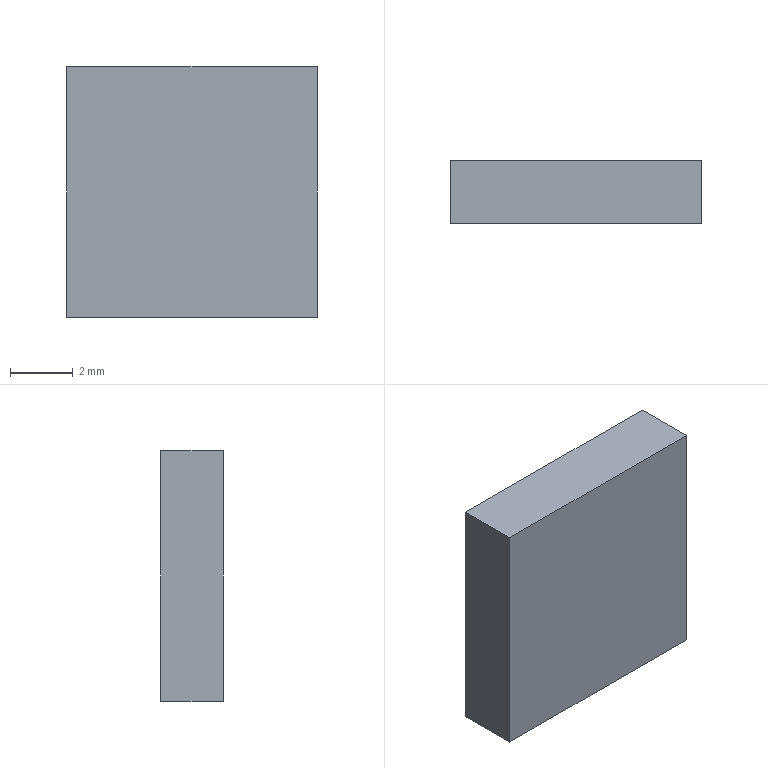Part | SolidWorks | features Extrusion 1 | 1 solid | 6 faces | box 8 x 2 x 8 mm | volume 128 mm3 | plane 6
STEP:
#1=CARTESIAN_POINT('',(4.,0.,4.));
#2=VERTEX_POINT('',#1);
#3=CARTESIAN_POINT('',(4.,0.,-4.));
#4=VERTEX_POINT('',#3);
#5=CARTESIAN_POINT('',(4.,0.,-4.));
#6=DIRECTION('',(0.,0.,-1.));
#7=VECTOR('',#6,1000.);
#8=LINE('',#5,#7);
#9=EDGE_CURVE('',#2,#4,#8,.T.);
#10=ORIENTED_EDGE('',*,*,#9,.T.);
#11=CARTESIAN_POINT('',(4.,2.,-4.));
#12=VERTEX_POINT('',#11);
#13=CARTESIAN_POINT('',(4.,2.,-4.));
#14=DIRECTION('',(0.,-1.,0.));
#15=VECTOR('',#14,1000.);
#16=LINE('',#13,#15);
#17=EDGE_CURVE('',#12,#4,#16,.T.);
#18=ORIENTED_EDGE('',*,*,#17,.F.);
#19=CARTESIAN_POINT('',(4.,2.,4.));
#20=VERTEX_POINT('',#19);
#21=CARTESIAN_POINT('',(4.,2.,-4.));
#22=DIRECTION('',(0.,0.,-1.));
#23=VECTOR('',#22,1000.);
#24=LINE('',#21,#23);
#25=EDGE_CURVE('',#20,#12,#24,.T.);
#26=ORIENTED_EDGE('',*,*,#25,.F.);
#27=CARTESIAN_POINT('',(4.,2.,4.));
#28=DIRECTION('',(0.,-1.,0.));
#29=VECTOR('',#28,1000.);
#30=LINE('',#27,#29);
#31=EDGE_CURVE('',#20,#2,#30,.T.);
#32=ORIENTED_EDGE('',*,*,#31,.T.);
#33=EDGE_LOOP('',(#10,#18,#26,#32));
#34=FACE_OUTER_BOUND('',#33,.T.);
#35=CARTESIAN_POINT('',(4.,2.,-4.));
#36=DIRECTION('',(-1.,0.,0.));
#37=DIRECTION('',(0.,0.,1.));
#38=AXIS2_PLACEMENT_3D('',#35,#36,#37);
#39=PLANE('',#38);
#40=ADVANCED_FACE('',(#34),#39,.F.);
#41=CARTESIAN_POINT('',(-4.,0.,-4.));
#42=VERTEX_POINT('',#41);
#43=CARTESIAN_POINT('',(-4.,0.,-4.));
#44=DIRECTION('',(-1.,0.,0.));
#45=VECTOR('',#44,1000.);
#46=LINE('',#43,#45);
#47=EDGE_CURVE('',#4,#42,#46,.T.);
#48=ORIENTED_EDGE('',*,*,#47,.T.);
#49=CARTESIAN_POINT('',(-4.,2.,-4.));
#50=VERTEX_POINT('',#49);
#51=CARTESIAN_POINT('',(-4.,2.,-4.));
#52=DIRECTION('',(0.,-1.,0.));
#53=VECTOR('',#52,1000.);
#54=LINE('',#51,#53);
#55=EDGE_CURVE('',#50,#42,#54,.T.);
#56=ORIENTED_EDGE('',*,*,#55,.F.);
#57=CARTESIAN_POINT('',(-4.,2.,-4.));
#58=DIRECTION('',(-1.,0.,0.));
#59=VECTOR('',#58,1000.);
#60=LINE('',#57,#59);
#61=EDGE_CURVE('',#12,#50,#60,.T.);
#62=ORIENTED_EDGE('',*,*,#61,.F.);
#63=ORIENTED_EDGE('',*,*,#17,.T.);
#64=EDGE_LOOP('',(#48,#56,#62,#63));
#65=FACE_OUTER_BOUND('',#64,.T.);
#66=CARTESIAN_POINT('',(-4.,2.,-4.));
#67=DIRECTION('',(0.,0.,1.));
#68=DIRECTION('',(1.,0.,0.));
#69=AXIS2_PLACEMENT_3D('',#66,#67,#68);
#70=PLANE('',#69);
#71=ADVANCED_FACE('',(#65),#70,.F.);
#72=CARTESIAN_POINT('',(-4.,0.,4.));
#73=VERTEX_POINT('',#72);
#74=CARTESIAN_POINT('',(-4.,0.,-4.));
#75=DIRECTION('',(0.,0.,1.));
#76=VECTOR('',#75,1000.);
#77=LINE('',#74,#76);
#78=EDGE_CURVE('',#42,#73,#77,.T.);
#79=ORIENTED_EDGE('',*,*,#78,.T.);
#80=CARTESIAN_POINT('',(-4.,2.,4.));
#81=VERTEX_POINT('',#80);
#82=CARTESIAN_POINT('',(-4.,2.,4.));
#83=DIRECTION('',(0.,-1.,0.));
#84=VECTOR('',#83,1000.);
#85=LINE('',#82,#84);
#86=EDGE_CURVE('',#81,#73,#85,.T.);
#87=ORIENTED_EDGE('',*,*,#86,.F.);
#88=CARTESIAN_POINT('',(-4.,2.,-4.));
#89=DIRECTION('',(0.,0.,1.));
#90=VECTOR('',#89,1000.);
#91=LINE('',#88,#90);
#92=EDGE_CURVE('',#50,#81,#91,.T.);
#93=ORIENTED_EDGE('',*,*,#92,.F.);
#94=ORIENTED_EDGE('',*,*,#55,.T.);
#95=EDGE_LOOP('',(#79,#87,#93,#94));
#96=FACE_OUTER_BOUND('',#95,.T.);
#97=CARTESIAN_POINT('',(-4.,2.,-4.));
#98=DIRECTION('',(1.,0.,0.));
#99=DIRECTION('',(0.,0.,-1.));
#100=AXIS2_PLACEMENT_3D('',#97,#98,#99);
#101=PLANE('',#100);
#102=ADVANCED_FACE('',(#96),#101,.F.);
#103=CARTESIAN_POINT('',(-4.,0.,4.));
#104=DIRECTION('',(1.,0.,0.));
#105=VECTOR('',#104,1000.);
#106=LINE('',#103,#105);
#107=EDGE_CURVE('',#73,#2,#106,.T.);
#108=ORIENTED_EDGE('',*,*,#107,.T.);
#109=ORIENTED_EDGE('',*,*,#31,.F.);
#110=CARTESIAN_POINT('',(-4.,2.,4.));
#111=DIRECTION('',(1.,0.,0.));
#112=VECTOR('',#111,1000.);
#113=LINE('',#110,#112);
#114=EDGE_CURVE('',#81,#20,#113,.T.);
#115=ORIENTED_EDGE('',*,*,#114,.F.);
#116=ORIENTED_EDGE('',*,*,#86,.T.);
#117=EDGE_LOOP('',(#108,#109,#115,#116));
#118=FACE_OUTER_BOUND('',#117,.T.);
#119=CARTESIAN_POINT('',(-4.,2.,4.));
#120=DIRECTION('',(0.,0.,-1.));
#121=DIRECTION('',(-1.,0.,0.));
#122=AXIS2_PLACEMENT_3D('',#119,#120,#121);
#123=PLANE('',#122);
#124=ADVANCED_FACE('',(#118),#123,.F.);
#125=ORIENTED_EDGE('',*,*,#25,.T.);
#126=ORIENTED_EDGE('',*,*,#61,.T.);
#127=ORIENTED_EDGE('',*,*,#92,.T.);
#128=ORIENTED_EDGE('',*,*,#114,.T.);
#129=EDGE_LOOP('',(#125,#126,#127,#128));
#130=FACE_OUTER_BOUND('',#129,.T.);
#131=CARTESIAN_POINT('',(0.,2.,0.));
#132=DIRECTION('',(0.,1.,0.));
#133=DIRECTION('',(0.,0.,1.));
#134=AXIS2_PLACEMENT_3D('',#131,#132,#133);
#135=PLANE('',#134);
#136=ADVANCED_FACE('',(#130),#135,.T.);
#137=ORIENTED_EDGE('',*,*,#9,.F.);
#138=ORIENTED_EDGE('',*,*,#107,.F.);
#139=ORIENTED_EDGE('',*,*,#78,.F.);
#140=ORIENTED_EDGE('',*,*,#47,.F.);
#141=EDGE_LOOP('',(#137,#138,#139,#140));
#142=FACE_OUTER_BOUND('',#141,.T.);
#143=CARTESIAN_POINT('',(0.,0.,0.));
#144=DIRECTION('',(0.,1.,0.));
#145=DIRECTION('',(0.,0.,1.));
#146=AXIS2_PLACEMENT_3D('',#143,#144,#145);
#147=PLANE('',#146);
#148=ADVANCED_FACE('',(#142),#147,.F.);
#149=CLOSED_SHELL('',(#40,#71,#102,#124,#136,#148));
#150=MANIFOLD_SOLID_BREP('',#149);
#151=CARTESIAN_POINT('',(0.,0.,0.));
#152=DIRECTION('',(0.,0.,1.));
#153=DIRECTION('',(1.,0.,0.));
#154=AXIS2_PLACEMENT_3D('',#151,#152,#153);
#155=(LENGTH_UNIT()NAMED_UNIT(*)SI_UNIT(.MILLI.,.METRE.));
#156=UNCERTAINTY_MEASURE_WITH_UNIT(LENGTH_MEASURE(0.00001),#155,'','');
#157=(NAMED_UNIT(*)PLANE_ANGLE_UNIT()SI_UNIT($,.RADIAN.));
#158=(NAMED_UNIT(*)SI_UNIT($,.STERADIAN.)SOLID_ANGLE_UNIT());
#159=(GEOMETRIC_REPRESENTATION_CONTEXT(3)GLOBAL_UNCERTAINTY_ASSIGNED_CONTEXT((#156))GLOBAL_UNIT_ASSIGNED_CONTEXT((#155,#157,#158))REPRESENTATION_CONTEXT('',''));
#160=ADVANCED_BREP_SHAPE_REPRESENTATION('',(#150,#154),#159);